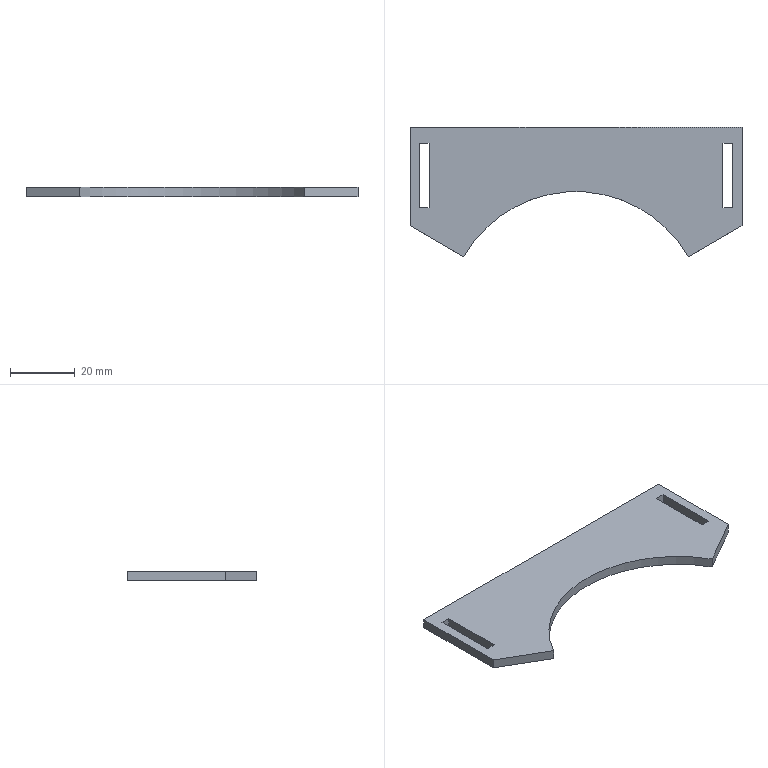Part | SolidWorks | features Extrusion 1, ICE 1 | 1 solid | 16 faces | box 102.9 x 40.212 x 3 mm | volume 8591 mm3 | plane 15 | cylinder 1 | commonest cylinder face diameters 80 x1
STEP:
#1=CARTESIAN_POINT('',(103.9,0.,3.));
#2=VERTEX_POINT('',#1);
#3=CARTESIAN_POINT('',(103.9,-30.577,3.));
#4=VERTEX_POINT('',#3);
#5=CARTESIAN_POINT('',(103.9,0.,3.));
#6=DIRECTION('',(0.,-1.,0.));
#7=VECTOR('',#6,1000.);
#8=LINE('',#5,#7);
#9=EDGE_CURVE('',#2,#4,#8,.T.);
#10=ORIENTED_EDGE('',*,*,#9,.F.);
#11=CARTESIAN_POINT('',(1.,0.,3.));
#12=VERTEX_POINT('',#11);
#13=CARTESIAN_POINT('',(0.,0.,3.));
#14=DIRECTION('',(-1.,0.,0.));
#15=VECTOR('',#14,1000.);
#16=LINE('',#13,#15);
#17=EDGE_CURVE('',#2,#12,#16,.T.);
#18=ORIENTED_EDGE('',*,*,#17,.T.);
#19=CARTESIAN_POINT('',(1.,-30.577,3.));
#20=VERTEX_POINT('',#19);
#21=CARTESIAN_POINT('',(1.,0.,3.));
#22=DIRECTION('',(0.,1.,0.));
#23=VECTOR('',#22,1000.);
#24=LINE('',#21,#23);
#25=EDGE_CURVE('',#20,#12,#24,.T.);
#26=ORIENTED_EDGE('',*,*,#25,.F.);
#27=CARTESIAN_POINT('',(17.688,-40.212,3.));
#28=VERTEX_POINT('',#27);
#29=CARTESIAN_POINT('',(0.,-30.,3.));
#30=DIRECTION('',(0.866,-0.5,0.));
#31=VECTOR('',#30,1000.);
#32=LINE('',#29,#31);
#33=EDGE_CURVE('',#20,#28,#32,.T.);
#34=ORIENTED_EDGE('',*,*,#33,.T.);
#35=CARTESIAN_POINT('',(87.212,-40.212,3.));
#36=VERTEX_POINT('',#35);
#37=CARTESIAN_POINT('',(52.45,-60.,3.));
#38=DIRECTION('',(0.,0.,-1.));
#39=DIRECTION('',(1.,0.,0.));
#40=AXIS2_PLACEMENT_3D('',#37,#38,#39);
#41=CIRCLE('',#40,40.);
#42=EDGE_CURVE('',#28,#36,#41,.T.);
#43=ORIENTED_EDGE('',*,*,#42,.T.);
#44=CARTESIAN_POINT('',(104.9,-30.,3.));
#45=DIRECTION('',(0.866,0.5,0.));
#46=VECTOR('',#45,1000.);
#47=LINE('',#44,#46);
#48=EDGE_CURVE('',#36,#4,#47,.T.);
#49=ORIENTED_EDGE('',*,*,#48,.T.);
#50=EDGE_LOOP('',(#10,#18,#26,#34,#43,#49));
#51=FACE_OUTER_BOUND('',#50,.T.);
#52=CARTESIAN_POINT('',(98.,-25.,3.));
#53=VERTEX_POINT('',#52);
#54=CARTESIAN_POINT('',(100.9,-25.,3.));
#55=VERTEX_POINT('',#54);
#56=CARTESIAN_POINT('',(98.,-25.,3.));
#57=DIRECTION('',(1.,0.,0.));
#58=VECTOR('',#57,1000.);
#59=LINE('',#56,#58);
#60=EDGE_CURVE('',#53,#55,#59,.T.);
#61=ORIENTED_EDGE('',*,*,#60,.F.);
#62=CARTESIAN_POINT('',(98.,-5.,3.));
#63=VERTEX_POINT('',#62);
#64=CARTESIAN_POINT('',(98.,-5.,3.));
#65=DIRECTION('',(0.,-1.,0.));
#66=VECTOR('',#65,1000.);
#67=LINE('',#64,#66);
#68=EDGE_CURVE('',#63,#53,#67,.T.);
#69=ORIENTED_EDGE('',*,*,#68,.F.);
#70=CARTESIAN_POINT('',(100.9,-5.,3.));
#71=VERTEX_POINT('',#70);
#72=CARTESIAN_POINT('',(98.,-5.,3.));
#73=DIRECTION('',(-1.,0.,0.));
#74=VECTOR('',#73,1000.);
#75=LINE('',#72,#74);
#76=EDGE_CURVE('',#71,#63,#75,.T.);
#77=ORIENTED_EDGE('',*,*,#76,.F.);
#78=CARTESIAN_POINT('',(100.9,-5.,3.));
#79=DIRECTION('',(0.,1.,0.));
#80=VECTOR('',#79,1000.);
#81=LINE('',#78,#80);
#82=EDGE_CURVE('',#55,#71,#81,.T.);
#83=ORIENTED_EDGE('',*,*,#82,.F.);
#84=EDGE_LOOP('',(#61,#69,#77,#83));
#85=FACE_BOUND('',#84,.T.);
#86=CARTESIAN_POINT('',(4.,-25.,3.));
#87=VERTEX_POINT('',#86);
#88=CARTESIAN_POINT('',(6.9,-25.,3.));
#89=VERTEX_POINT('',#88);
#90=CARTESIAN_POINT('',(4.,-25.,3.));
#91=DIRECTION('',(1.,0.,0.));
#92=VECTOR('',#91,1000.);
#93=LINE('',#90,#92);
#94=EDGE_CURVE('',#87,#89,#93,.T.);
#95=ORIENTED_EDGE('',*,*,#94,.F.);
#96=CARTESIAN_POINT('',(4.,-5.,3.));
#97=VERTEX_POINT('',#96);
#98=CARTESIAN_POINT('',(4.,-5.,3.));
#99=DIRECTION('',(0.,-1.,0.));
#100=VECTOR('',#99,1000.);
#101=LINE('',#98,#100);
#102=EDGE_CURVE('',#97,#87,#101,.T.);
#103=ORIENTED_EDGE('',*,*,#102,.F.);
#104=CARTESIAN_POINT('',(6.9,-5.,3.));
#105=VERTEX_POINT('',#104);
#106=CARTESIAN_POINT('',(4.,-5.,3.));
#107=DIRECTION('',(-1.,0.,0.));
#108=VECTOR('',#107,1000.);
#109=LINE('',#106,#108);
#110=EDGE_CURVE('',#105,#97,#109,.T.);
#111=ORIENTED_EDGE('',*,*,#110,.F.);
#112=CARTESIAN_POINT('',(6.9,-5.,3.));
#113=DIRECTION('',(0.,1.,0.));
#114=VECTOR('',#113,1000.);
#115=LINE('',#112,#114);
#116=EDGE_CURVE('',#89,#105,#115,.T.);
#117=ORIENTED_EDGE('',*,*,#116,.F.);
#118=EDGE_LOOP('',(#95,#103,#111,#117));
#119=FACE_BOUND('',#118,.T.);
#120=CARTESIAN_POINT('',(52.45,-60.,3.));
#121=DIRECTION('',(0.,0.,1.));
#122=DIRECTION('',(1.,0.,0.));
#123=AXIS2_PLACEMENT_3D('',#120,#121,#122);
#124=PLANE('',#123);
#125=ADVANCED_FACE('',(#51,#85,#119),#124,.T.);
#126=CARTESIAN_POINT('',(98.,-5.,0.));
#127=VERTEX_POINT('',#126);
#128=CARTESIAN_POINT('',(98.,-25.,0.));
#129=VERTEX_POINT('',#128);
#130=CARTESIAN_POINT('',(98.,-5.,0.));
#131=DIRECTION('',(0.,-1.,0.));
#132=VECTOR('',#131,1000.);
#133=LINE('',#130,#132);
#134=EDGE_CURVE('',#127,#129,#133,.T.);
#135=ORIENTED_EDGE('',*,*,#134,.T.);
#136=CARTESIAN_POINT('',(100.9,-25.,0.));
#137=VERTEX_POINT('',#136);
#138=CARTESIAN_POINT('',(98.,-25.,0.));
#139=DIRECTION('',(1.,0.,0.));
#140=VECTOR('',#139,1000.);
#141=LINE('',#138,#140);
#142=EDGE_CURVE('',#129,#137,#141,.T.);
#143=ORIENTED_EDGE('',*,*,#142,.T.);
#144=CARTESIAN_POINT('',(100.9,-5.,0.));
#145=VERTEX_POINT('',#144);
#146=CARTESIAN_POINT('',(100.9,-5.,0.));
#147=DIRECTION('',(0.,1.,0.));
#148=VECTOR('',#147,1000.);
#149=LINE('',#146,#148);
#150=EDGE_CURVE('',#137,#145,#149,.T.);
#151=ORIENTED_EDGE('',*,*,#150,.T.);
#152=CARTESIAN_POINT('',(98.,-5.,0.));
#153=DIRECTION('',(-1.,0.,0.));
#154=VECTOR('',#153,1000.);
#155=LINE('',#152,#154);
#156=EDGE_CURVE('',#145,#127,#155,.T.);
#157=ORIENTED_EDGE('',*,*,#156,.T.);
#158=EDGE_LOOP('',(#135,#143,#151,#157));
#159=FACE_BOUND('',#158,.T.);
#160=CARTESIAN_POINT('',(103.9,0.,0.));
#161=VERTEX_POINT('',#160);
#162=CARTESIAN_POINT('',(1.,0.,0.));
#163=VERTEX_POINT('',#162);
#164=CARTESIAN_POINT('',(0.,0.,0.));
#165=DIRECTION('',(-1.,0.,0.));
#166=VECTOR('',#165,1000.);
#167=LINE('',#164,#166);
#168=EDGE_CURVE('',#161,#163,#167,.T.);
#169=ORIENTED_EDGE('',*,*,#168,.F.);
#170=CARTESIAN_POINT('',(103.9,-30.577,0.));
#171=VERTEX_POINT('',#170);
#172=CARTESIAN_POINT('',(103.9,0.,0.));
#173=DIRECTION('',(0.,-1.,0.));
#174=VECTOR('',#173,1000.);
#175=LINE('',#172,#174);
#176=EDGE_CURVE('',#161,#171,#175,.T.);
#177=ORIENTED_EDGE('',*,*,#176,.T.);
#178=CARTESIAN_POINT('',(87.212,-40.212,0.));
#179=VERTEX_POINT('',#178);
#180=CARTESIAN_POINT('',(104.9,-30.,0.));
#181=DIRECTION('',(0.866,0.5,0.));
#182=VECTOR('',#181,1000.);
#183=LINE('',#180,#182);
#184=EDGE_CURVE('',#179,#171,#183,.T.);
#185=ORIENTED_EDGE('',*,*,#184,.F.);
#186=CARTESIAN_POINT('',(17.688,-40.212,0.));
#187=VERTEX_POINT('',#186);
#188=CARTESIAN_POINT('',(52.45,-60.,0.));
#189=DIRECTION('',(0.,0.,-1.));
#190=DIRECTION('',(1.,0.,0.));
#191=AXIS2_PLACEMENT_3D('',#188,#189,#190);
#192=CIRCLE('',#191,40.);
#193=EDGE_CURVE('',#187,#179,#192,.T.);
#194=ORIENTED_EDGE('',*,*,#193,.F.);
#195=CARTESIAN_POINT('',(1.,-30.577,0.));
#196=VERTEX_POINT('',#195);
#197=CARTESIAN_POINT('',(0.,-30.,0.));
#198=DIRECTION('',(0.866,-0.5,0.));
#199=VECTOR('',#198,1000.);
#200=LINE('',#197,#199);
#201=EDGE_CURVE('',#196,#187,#200,.T.);
#202=ORIENTED_EDGE('',*,*,#201,.F.);
#203=CARTESIAN_POINT('',(1.,0.,0.));
#204=DIRECTION('',(0.,1.,0.));
#205=VECTOR('',#204,1000.);
#206=LINE('',#203,#205);
#207=EDGE_CURVE('',#196,#163,#206,.T.);
#208=ORIENTED_EDGE('',*,*,#207,.T.);
#209=EDGE_LOOP('',(#169,#177,#185,#194,#202,#208));
#210=FACE_OUTER_BOUND('',#209,.T.);
#211=CARTESIAN_POINT('',(4.,-5.,0.));
#212=VERTEX_POINT('',#211);
#213=CARTESIAN_POINT('',(4.,-25.,0.));
#214=VERTEX_POINT('',#213);
#215=CARTESIAN_POINT('',(4.,-5.,0.));
#216=DIRECTION('',(0.,-1.,0.));
#217=VECTOR('',#216,1000.);
#218=LINE('',#215,#217);
#219=EDGE_CURVE('',#212,#214,#218,.T.);
#220=ORIENTED_EDGE('',*,*,#219,.T.);
#221=CARTESIAN_POINT('',(6.9,-25.,0.));
#222=VERTEX_POINT('',#221);
#223=CARTESIAN_POINT('',(4.,-25.,0.));
#224=DIRECTION('',(1.,0.,0.));
#225=VECTOR('',#224,1000.);
#226=LINE('',#223,#225);
#227=EDGE_CURVE('',#214,#222,#226,.T.);
#228=ORIENTED_EDGE('',*,*,#227,.T.);
#229=CARTESIAN_POINT('',(6.9,-5.,0.));
#230=VERTEX_POINT('',#229);
#231=CARTESIAN_POINT('',(6.9,-5.,0.));
#232=DIRECTION('',(0.,1.,0.));
#233=VECTOR('',#232,1000.);
#234=LINE('',#231,#233);
#235=EDGE_CURVE('',#222,#230,#234,.T.);
#236=ORIENTED_EDGE('',*,*,#235,.T.);
#237=CARTESIAN_POINT('',(4.,-5.,0.));
#238=DIRECTION('',(-1.,0.,0.));
#239=VECTOR('',#238,1000.);
#240=LINE('',#237,#239);
#241=EDGE_CURVE('',#230,#212,#240,.T.);
#242=ORIENTED_EDGE('',*,*,#241,.T.);
#243=EDGE_LOOP('',(#220,#228,#236,#242));
#244=FACE_BOUND('',#243,.T.);
#245=CARTESIAN_POINT('',(52.45,-60.,0.));
#246=DIRECTION('',(0.,0.,1.));
#247=DIRECTION('',(1.,0.,0.));
#248=AXIS2_PLACEMENT_3D('',#245,#246,#247);
#249=PLANE('',#248);
#250=ADVANCED_FACE('',(#159,#210,#244),#249,.F.);
#251=ORIENTED_EDGE('',*,*,#33,.F.);
#252=CARTESIAN_POINT('',(1.,-30.577,0.));
#253=DIRECTION('',(0.,0.,1.));
#254=VECTOR('',#253,1000.);
#255=LINE('',#252,#254);
#256=EDGE_CURVE('',#196,#20,#255,.T.);
#257=ORIENTED_EDGE('',*,*,#256,.F.);
#258=ORIENTED_EDGE('',*,*,#201,.T.);
#259=CARTESIAN_POINT('',(17.688,-40.212,3.));
#260=DIRECTION('',(0.,0.,-1.));
#261=VECTOR('',#260,1000.);
#262=LINE('',#259,#261);
#263=EDGE_CURVE('',#28,#187,#262,.T.);
#264=ORIENTED_EDGE('',*,*,#263,.F.);
#265=EDGE_LOOP('',(#251,#257,#258,#264));
#266=FACE_OUTER_BOUND('',#265,.T.);
#267=CARTESIAN_POINT('',(0.,-30.,3.));
#268=DIRECTION('',(0.5,0.866,0.));
#269=DIRECTION('',(-0.866,0.5,0.));
#270=AXIS2_PLACEMENT_3D('',#267,#268,#269);
#271=PLANE('',#270);
#272=ADVANCED_FACE('',(#266),#271,.F.);
#273=ORIENTED_EDGE('',*,*,#193,.T.);
#274=CARTESIAN_POINT('',(87.212,-40.212,3.));
#275=DIRECTION('',(0.,0.,-1.));
#276=VECTOR('',#275,1000.);
#277=LINE('',#274,#276);
#278=EDGE_CURVE('',#36,#179,#277,.T.);
#279=ORIENTED_EDGE('',*,*,#278,.F.);
#280=ORIENTED_EDGE('',*,*,#42,.F.);
#281=ORIENTED_EDGE('',*,*,#263,.T.);
#282=EDGE_LOOP('',(#273,#279,#280,#281));
#283=FACE_OUTER_BOUND('',#282,.T.);
#284=CARTESIAN_POINT('',(52.45,-60.,3.));
#285=DIRECTION('',(0.,0.,-1.));
#286=DIRECTION('',(-1.,0.,0.));
#287=AXIS2_PLACEMENT_3D('',#284,#285,#286);
#288=CYLINDRICAL_SURFACE('',#287,40.);
#289=ADVANCED_FACE('',(#283),#288,.F.);
#290=ORIENTED_EDGE('',*,*,#184,.T.);
#291=CARTESIAN_POINT('',(103.9,-30.577,0.));
#292=DIRECTION('',(0.,0.,1.));
#293=VECTOR('',#292,1000.);
#294=LINE('',#291,#293);
#295=EDGE_CURVE('',#171,#4,#294,.T.);
#296=ORIENTED_EDGE('',*,*,#295,.T.);
#297=ORIENTED_EDGE('',*,*,#48,.F.);
#298=ORIENTED_EDGE('',*,*,#278,.T.);
#299=EDGE_LOOP('',(#290,#296,#297,#298));
#300=FACE_OUTER_BOUND('',#299,.T.);
#301=CARTESIAN_POINT('',(104.9,-30.,3.));
#302=DIRECTION('',(-0.5,0.866,0.));
#303=DIRECTION('',(-0.866,-0.5,0.));
#304=AXIS2_PLACEMENT_3D('',#301,#302,#303);
#305=PLANE('',#304);
#306=ADVANCED_FACE('',(#300),#305,.F.);
#307=ORIENTED_EDGE('',*,*,#17,.F.);
#308=CARTESIAN_POINT('',(103.9,0.,0.));
#309=DIRECTION('',(0.,0.,1.));
#310=VECTOR('',#309,1000.);
#311=LINE('',#308,#310);
#312=EDGE_CURVE('',#161,#2,#311,.T.);
#313=ORIENTED_EDGE('',*,*,#312,.F.);
#314=ORIENTED_EDGE('',*,*,#168,.T.);
#315=CARTESIAN_POINT('',(1.,0.,0.));
#316=DIRECTION('',(0.,0.,1.));
#317=VECTOR('',#316,1000.);
#318=LINE('',#315,#317);
#319=EDGE_CURVE('',#163,#12,#318,.T.);
#320=ORIENTED_EDGE('',*,*,#319,.T.);
#321=EDGE_LOOP('',(#307,#313,#314,#320));
#322=FACE_OUTER_BOUND('',#321,.T.);
#323=CARTESIAN_POINT('',(0.,0.,3.));
#324=DIRECTION('',(0.,-1.,0.));
#325=DIRECTION('',(0.,0.,-1.));
#326=AXIS2_PLACEMENT_3D('',#323,#324,#325);
#327=PLANE('',#326);
#328=ADVANCED_FACE('',(#322),#327,.F.);
#329=ORIENTED_EDGE('',*,*,#134,.F.);
#330=CARTESIAN_POINT('',(98.,-5.,3.));
#331=DIRECTION('',(0.,0.,-1.));
#332=VECTOR('',#331,1000.);
#333=LINE('',#330,#332);
#334=EDGE_CURVE('',#63,#127,#333,.T.);
#335=ORIENTED_EDGE('',*,*,#334,.F.);
#336=ORIENTED_EDGE('',*,*,#68,.T.);
#337=CARTESIAN_POINT('',(98.,-25.,3.));
#338=DIRECTION('',(0.,0.,-1.));
#339=VECTOR('',#338,1000.);
#340=LINE('',#337,#339);
#341=EDGE_CURVE('',#53,#129,#340,.T.);
#342=ORIENTED_EDGE('',*,*,#341,.T.);
#343=EDGE_LOOP('',(#329,#335,#336,#342));
#344=FACE_OUTER_BOUND('',#343,.T.);
#345=CARTESIAN_POINT('',(98.,-5.,3.));
#346=DIRECTION('',(1.,0.,0.));
#347=DIRECTION('',(0.,0.,-1.));
#348=AXIS2_PLACEMENT_3D('',#345,#346,#347);
#349=PLANE('',#348);
#350=ADVANCED_FACE('',(#344),#349,.T.);
#351=ORIENTED_EDGE('',*,*,#142,.F.);
#352=ORIENTED_EDGE('',*,*,#341,.F.);
#353=ORIENTED_EDGE('',*,*,#60,.T.);
#354=CARTESIAN_POINT('',(100.9,-25.,3.));
#355=DIRECTION('',(0.,0.,-1.));
#356=VECTOR('',#355,1000.);
#357=LINE('',#354,#356);
#358=EDGE_CURVE('',#55,#137,#357,.T.);
#359=ORIENTED_EDGE('',*,*,#358,.T.);
#360=EDGE_LOOP('',(#351,#352,#353,#359));
#361=FACE_OUTER_BOUND('',#360,.T.);
#362=CARTESIAN_POINT('',(98.,-25.,3.));
#363=DIRECTION('',(0.,1.,0.));
#364=DIRECTION('',(0.,0.,1.));
#365=AXIS2_PLACEMENT_3D('',#362,#363,#364);
#366=PLANE('',#365);
#367=ADVANCED_FACE('',(#361),#366,.T.);
#368=ORIENTED_EDGE('',*,*,#150,.F.);
#369=ORIENTED_EDGE('',*,*,#358,.F.);
#370=ORIENTED_EDGE('',*,*,#82,.T.);
#371=CARTESIAN_POINT('',(100.9,-5.,3.));
#372=DIRECTION('',(0.,0.,-1.));
#373=VECTOR('',#372,1000.);
#374=LINE('',#371,#373);
#375=EDGE_CURVE('',#71,#145,#374,.T.);
#376=ORIENTED_EDGE('',*,*,#375,.T.);
#377=EDGE_LOOP('',(#368,#369,#370,#376));
#378=FACE_OUTER_BOUND('',#377,.T.);
#379=CARTESIAN_POINT('',(100.9,-5.,3.));
#380=DIRECTION('',(-1.,0.,0.));
#381=DIRECTION('',(0.,0.,1.));
#382=AXIS2_PLACEMENT_3D('',#379,#380,#381);
#383=PLANE('',#382);
#384=ADVANCED_FACE('',(#378),#383,.T.);
#385=ORIENTED_EDGE('',*,*,#156,.F.);
#386=ORIENTED_EDGE('',*,*,#375,.F.);
#387=ORIENTED_EDGE('',*,*,#76,.T.);
#388=ORIENTED_EDGE('',*,*,#334,.T.);
#389=EDGE_LOOP('',(#385,#386,#387,#388));
#390=FACE_OUTER_BOUND('',#389,.T.);
#391=CARTESIAN_POINT('',(98.,-5.,3.));
#392=DIRECTION('',(0.,-1.,0.));
#393=DIRECTION('',(0.,0.,-1.));
#394=AXIS2_PLACEMENT_3D('',#391,#392,#393);
#395=PLANE('',#394);
#396=ADVANCED_FACE('',(#390),#395,.T.);
#397=ORIENTED_EDGE('',*,*,#219,.F.);
#398=CARTESIAN_POINT('',(4.,-5.,3.));
#399=DIRECTION('',(0.,0.,-1.));
#400=VECTOR('',#399,1000.);
#401=LINE('',#398,#400);
#402=EDGE_CURVE('',#97,#212,#401,.T.);
#403=ORIENTED_EDGE('',*,*,#402,.F.);
#404=ORIENTED_EDGE('',*,*,#102,.T.);
#405=CARTESIAN_POINT('',(4.,-25.,3.));
#406=DIRECTION('',(0.,0.,-1.));
#407=VECTOR('',#406,1000.);
#408=LINE('',#405,#407);
#409=EDGE_CURVE('',#87,#214,#408,.T.);
#410=ORIENTED_EDGE('',*,*,#409,.T.);
#411=EDGE_LOOP('',(#397,#403,#404,#410));
#412=FACE_OUTER_BOUND('',#411,.T.);
#413=CARTESIAN_POINT('',(4.,-5.,3.));
#414=DIRECTION('',(1.,0.,0.));
#415=DIRECTION('',(0.,1.,0.));
#416=AXIS2_PLACEMENT_3D('',#413,#414,#415);
#417=PLANE('',#416);
#418=ADVANCED_FACE('',(#412),#417,.T.);
#419=ORIENTED_EDGE('',*,*,#227,.F.);
#420=ORIENTED_EDGE('',*,*,#409,.F.);
#421=ORIENTED_EDGE('',*,*,#94,.T.);
#422=CARTESIAN_POINT('',(6.9,-25.,3.));
#423=DIRECTION('',(0.,0.,-1.));
#424=VECTOR('',#423,1000.);
#425=LINE('',#422,#424);
#426=EDGE_CURVE('',#89,#222,#425,.T.);
#427=ORIENTED_EDGE('',*,*,#426,.T.);
#428=EDGE_LOOP('',(#419,#420,#421,#427));
#429=FACE_OUTER_BOUND('',#428,.T.);
#430=CARTESIAN_POINT('',(4.,-25.,3.));
#431=DIRECTION('',(0.,1.,0.));
#432=DIRECTION('',(-1.,0.,0.));
#433=AXIS2_PLACEMENT_3D('',#430,#431,#432);
#434=PLANE('',#433);
#435=ADVANCED_FACE('',(#429),#434,.T.);
#436=ORIENTED_EDGE('',*,*,#235,.F.);
#437=ORIENTED_EDGE('',*,*,#426,.F.);
#438=ORIENTED_EDGE('',*,*,#116,.T.);
#439=CARTESIAN_POINT('',(6.9,-5.,3.));
#440=DIRECTION('',(0.,0.,-1.));
#441=VECTOR('',#440,1000.);
#442=LINE('',#439,#441);
#443=EDGE_CURVE('',#105,#230,#442,.T.);
#444=ORIENTED_EDGE('',*,*,#443,.T.);
#445=EDGE_LOOP('',(#436,#437,#438,#444));
#446=FACE_OUTER_BOUND('',#445,.T.);
#447=CARTESIAN_POINT('',(6.9,-5.,3.));
#448=DIRECTION('',(-1.,0.,0.));
#449=DIRECTION('',(0.,-1.,0.));
#450=AXIS2_PLACEMENT_3D('',#447,#448,#449);
#451=PLANE('',#450);
#452=ADVANCED_FACE('',(#446),#451,.T.);
#453=ORIENTED_EDGE('',*,*,#241,.F.);
#454=ORIENTED_EDGE('',*,*,#443,.F.);
#455=ORIENTED_EDGE('',*,*,#110,.T.);
#456=ORIENTED_EDGE('',*,*,#402,.T.);
#457=EDGE_LOOP('',(#453,#454,#455,#456));
#458=FACE_OUTER_BOUND('',#457,.T.);
#459=CARTESIAN_POINT('',(4.,-5.,3.));
#460=DIRECTION('',(0.,-1.,0.));
#461=DIRECTION('',(0.,0.,-1.));
#462=AXIS2_PLACEMENT_3D('',#459,#460,#461);
#463=PLANE('',#462);
#464=ADVANCED_FACE('',(#458),#463,.T.);
#465=ORIENTED_EDGE('',*,*,#25,.T.);
#466=ORIENTED_EDGE('',*,*,#319,.F.);
#467=ORIENTED_EDGE('',*,*,#207,.F.);
#468=ORIENTED_EDGE('',*,*,#256,.T.);
#469=EDGE_LOOP('',(#465,#466,#467,#468));
#470=FACE_OUTER_BOUND('',#469,.T.);
#471=CARTESIAN_POINT('',(1.,0.,0.));
#472=DIRECTION('',(1.,0.,0.));
#473=DIRECTION('',(0.,1.,0.));
#474=AXIS2_PLACEMENT_3D('',#471,#472,#473);
#475=PLANE('',#474);
#476=ADVANCED_FACE('',(#470),#475,.F.);
#477=ORIENTED_EDGE('',*,*,#9,.T.);
#478=ORIENTED_EDGE('',*,*,#295,.F.);
#479=ORIENTED_EDGE('',*,*,#176,.F.);
#480=ORIENTED_EDGE('',*,*,#312,.T.);
#481=EDGE_LOOP('',(#477,#478,#479,#480));
#482=FACE_OUTER_BOUND('',#481,.T.);
#483=CARTESIAN_POINT('',(103.9,0.,0.));
#484=DIRECTION('',(-1.,0.,0.));
#485=DIRECTION('',(0.,0.,1.));
#486=AXIS2_PLACEMENT_3D('',#483,#484,#485);
#487=PLANE('',#486);
#488=ADVANCED_FACE('',(#482),#487,.F.);
#489=CLOSED_SHELL('',(#125,#250,#272,#289,#306,#328,#350,#367,#384,#396,#418,#435,#452,#464,#476,#488));
#490=MANIFOLD_SOLID_BREP('',#489);
#491=CARTESIAN_POINT('',(0.,0.,0.));
#492=DIRECTION('',(0.,0.,1.));
#493=DIRECTION('',(1.,0.,0.));
#494=AXIS2_PLACEMENT_3D('',#491,#492,#493);
#495=(LENGTH_UNIT()NAMED_UNIT(*)SI_UNIT(.MILLI.,.METRE.));
#496=UNCERTAINTY_MEASURE_WITH_UNIT(LENGTH_MEASURE(0.00001),#495,'','');
#497=(NAMED_UNIT(*)PLANE_ANGLE_UNIT()SI_UNIT($,.RADIAN.));
#498=(NAMED_UNIT(*)SI_UNIT($,.STERADIAN.)SOLID_ANGLE_UNIT());
#499=(GEOMETRIC_REPRESENTATION_CONTEXT(3)GLOBAL_UNCERTAINTY_ASSIGNED_CONTEXT((#496))GLOBAL_UNIT_ASSIGNED_CONTEXT((#495,#497,#498))REPRESENTATION_CONTEXT('',''));
#500=ADVANCED_BREP_SHAPE_REPRESENTATION('',(#490,#494),#499);